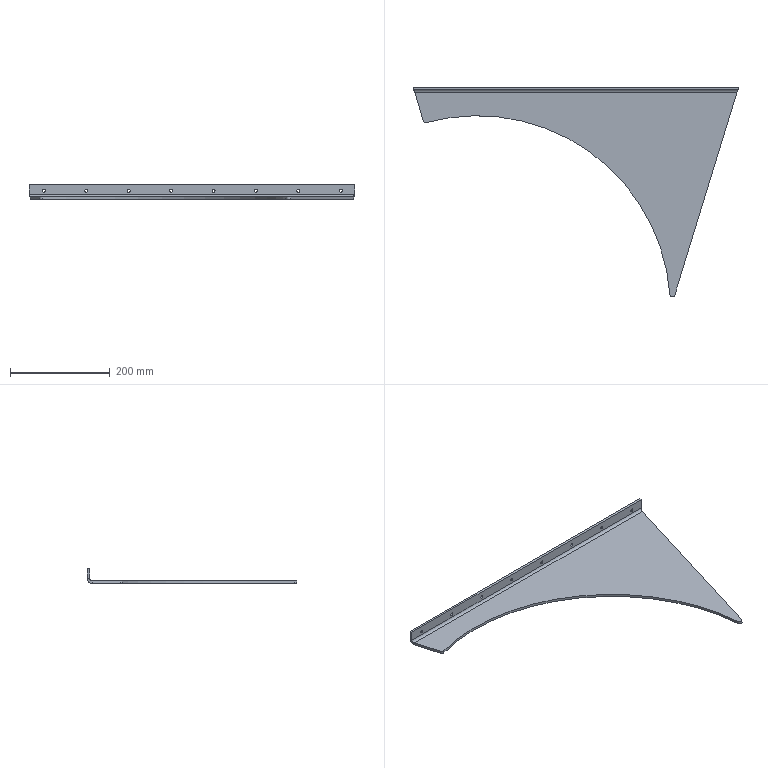Part | SolidWorks | features EdgeFlange 1, Fillet 1, FlatPattern 1, HoleWzd 1, LPattern 1, SMBaseFlange 1, SheetMetal 1 | 1 solid | 48 faces | box 651.256 x 419.882 x 30 mm | volume 529249 mm3 | cylinder 21 | cone 16 | plane 9 | spline 2 | commonest cylinder face diameters 6 x16 10 x3 20 x1 775 x1